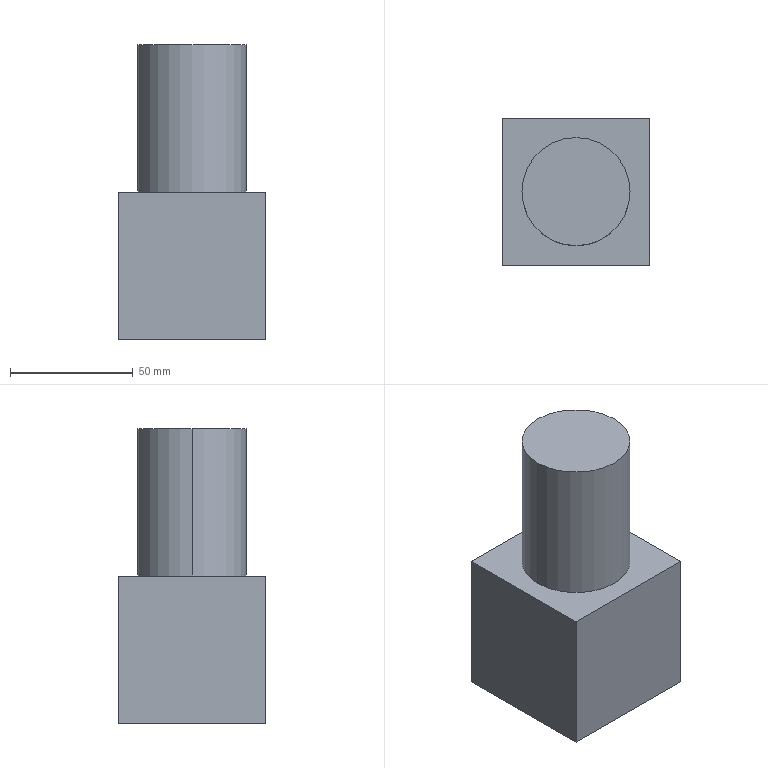Part | SolidWorks | features Extrusion 1, ICE 1 | 1 solid | 9 faces | box 60 x 60 x 120 mm | volume 307105 mm3 | plane 7 | cylinder 2 | commonest cylinder face diameters 43.97 x2
STEP:
#1=CARTESIAN_POINT('',(21.985,30.,90.));
#2=VERTEX_POINT('',#1);
#3=CARTESIAN_POINT('',(-21.985,30.,90.));
#4=VERTEX_POINT('',#3);
#5=CARTESIAN_POINT('',(0.,30.,90.));
#6=DIRECTION('',(0.,0.,1.));
#7=DIRECTION('',(1.,0.,0.));
#8=AXIS2_PLACEMENT_3D('',#5,#6,#7);
#9=CIRCLE('',#8,21.985);
#10=EDGE_CURVE('',#2,#4,#9,.T.);
#11=ORIENTED_EDGE('',*,*,#10,.F.);
#12=CARTESIAN_POINT('',(21.985,30.,30.));
#13=VERTEX_POINT('',#12);
#14=CARTESIAN_POINT('',(21.985,30.,90.));
#15=DIRECTION('',(0.,0.,-1.));
#16=VECTOR('',#15,1000.);
#17=LINE('',#14,#16);
#18=EDGE_CURVE('',#2,#13,#17,.T.);
#19=ORIENTED_EDGE('',*,*,#18,.T.);
#20=CARTESIAN_POINT('',(-21.985,30.,30.));
#21=VERTEX_POINT('',#20);
#22=CARTESIAN_POINT('',(0.,30.,30.));
#23=DIRECTION('',(0.,0.,1.));
#24=DIRECTION('',(1.,0.,0.));
#25=AXIS2_PLACEMENT_3D('',#22,#23,#24);
#26=CIRCLE('',#25,21.985);
#27=EDGE_CURVE('',#13,#21,#26,.T.);
#28=ORIENTED_EDGE('',*,*,#27,.T.);
#29=CARTESIAN_POINT('',(-21.985,30.,90.));
#30=DIRECTION('',(0.,0.,-1.));
#31=VECTOR('',#30,1000.);
#32=LINE('',#29,#31);
#33=EDGE_CURVE('',#4,#21,#32,.T.);
#34=ORIENTED_EDGE('',*,*,#33,.F.);
#35=EDGE_LOOP('',(#11,#19,#28,#34));
#36=FACE_OUTER_BOUND('',#35,.T.);
#37=CARTESIAN_POINT('',(0.,30.,90.));
#38=DIRECTION('',(0.,0.,-1.));
#39=DIRECTION('',(-1.,0.,0.));
#40=AXIS2_PLACEMENT_3D('',#37,#38,#39);
#41=CYLINDRICAL_SURFACE('',#40,21.985);
#42=ADVANCED_FACE('',(#36),#41,.T.);
#43=CARTESIAN_POINT('',(30.,0.,30.));
#44=VERTEX_POINT('',#43);
#45=CARTESIAN_POINT('',(30.,0.,-30.));
#46=VERTEX_POINT('',#45);
#47=CARTESIAN_POINT('',(30.,0.,-30.));
#48=DIRECTION('',(0.,0.,-1.));
#49=VECTOR('',#48,1000.);
#50=LINE('',#47,#49);
#51=EDGE_CURVE('',#44,#46,#50,.T.);
#52=ORIENTED_EDGE('',*,*,#51,.T.);
#53=CARTESIAN_POINT('',(30.,60.,-30.));
#54=VERTEX_POINT('',#53);
#55=CARTESIAN_POINT('',(30.,60.,-30.));
#56=DIRECTION('',(0.,-1.,0.));
#57=VECTOR('',#56,1000.);
#58=LINE('',#55,#57);
#59=EDGE_CURVE('',#54,#46,#58,.T.);
#60=ORIENTED_EDGE('',*,*,#59,.F.);
#61=CARTESIAN_POINT('',(30.,60.,30.));
#62=VERTEX_POINT('',#61);
#63=CARTESIAN_POINT('',(30.,60.,-30.));
#64=DIRECTION('',(0.,0.,-1.));
#65=VECTOR('',#64,1000.);
#66=LINE('',#63,#65);
#67=EDGE_CURVE('',#62,#54,#66,.T.);
#68=ORIENTED_EDGE('',*,*,#67,.F.);
#69=CARTESIAN_POINT('',(30.,60.,30.));
#70=DIRECTION('',(0.,-1.,0.));
#71=VECTOR('',#70,1000.);
#72=LINE('',#69,#71);
#73=EDGE_CURVE('',#62,#44,#72,.T.);
#74=ORIENTED_EDGE('',*,*,#73,.T.);
#75=EDGE_LOOP('',(#52,#60,#68,#74));
#76=FACE_OUTER_BOUND('',#75,.T.);
#77=CARTESIAN_POINT('',(30.,60.,-30.));
#78=DIRECTION('',(-1.,0.,0.));
#79=DIRECTION('',(0.,0.,1.));
#80=AXIS2_PLACEMENT_3D('',#77,#78,#79);
#81=PLANE('',#80);
#82=ADVANCED_FACE('',(#76),#81,.F.);
#83=CARTESIAN_POINT('',(-30.,0.,-30.));
#84=VERTEX_POINT('',#83);
#85=CARTESIAN_POINT('',(-30.,0.,-30.));
#86=DIRECTION('',(-1.,0.,0.));
#87=VECTOR('',#86,1000.);
#88=LINE('',#85,#87);
#89=EDGE_CURVE('',#46,#84,#88,.T.);
#90=ORIENTED_EDGE('',*,*,#89,.T.);
#91=CARTESIAN_POINT('',(-30.,60.,-30.));
#92=VERTEX_POINT('',#91);
#93=CARTESIAN_POINT('',(-30.,60.,-30.));
#94=DIRECTION('',(0.,-1.,0.));
#95=VECTOR('',#94,1000.);
#96=LINE('',#93,#95);
#97=EDGE_CURVE('',#92,#84,#96,.T.);
#98=ORIENTED_EDGE('',*,*,#97,.F.);
#99=CARTESIAN_POINT('',(-30.,60.,-30.));
#100=DIRECTION('',(-1.,0.,0.));
#101=VECTOR('',#100,1000.);
#102=LINE('',#99,#101);
#103=EDGE_CURVE('',#54,#92,#102,.T.);
#104=ORIENTED_EDGE('',*,*,#103,.F.);
#105=ORIENTED_EDGE('',*,*,#59,.T.);
#106=EDGE_LOOP('',(#90,#98,#104,#105));
#107=FACE_OUTER_BOUND('',#106,.T.);
#108=CARTESIAN_POINT('',(-30.,60.,-30.));
#109=DIRECTION('',(0.,0.,1.));
#110=DIRECTION('',(1.,0.,0.));
#111=AXIS2_PLACEMENT_3D('',#108,#109,#110);
#112=PLANE('',#111);
#113=ADVANCED_FACE('',(#107),#112,.F.);
#114=CARTESIAN_POINT('',(-30.,0.,30.));
#115=VERTEX_POINT('',#114);
#116=CARTESIAN_POINT('',(-30.,0.,-30.));
#117=DIRECTION('',(0.,0.,1.));
#118=VECTOR('',#117,1000.);
#119=LINE('',#116,#118);
#120=EDGE_CURVE('',#84,#115,#119,.T.);
#121=ORIENTED_EDGE('',*,*,#120,.T.);
#122=CARTESIAN_POINT('',(-30.,60.,30.));
#123=VERTEX_POINT('',#122);
#124=CARTESIAN_POINT('',(-30.,60.,30.));
#125=DIRECTION('',(0.,-1.,0.));
#126=VECTOR('',#125,1000.);
#127=LINE('',#124,#126);
#128=EDGE_CURVE('',#123,#115,#127,.T.);
#129=ORIENTED_EDGE('',*,*,#128,.F.);
#130=CARTESIAN_POINT('',(-30.,60.,-30.));
#131=DIRECTION('',(0.,0.,1.));
#132=VECTOR('',#131,1000.);
#133=LINE('',#130,#132);
#134=EDGE_CURVE('',#92,#123,#133,.T.);
#135=ORIENTED_EDGE('',*,*,#134,.F.);
#136=ORIENTED_EDGE('',*,*,#97,.T.);
#137=EDGE_LOOP('',(#121,#129,#135,#136));
#138=FACE_OUTER_BOUND('',#137,.T.);
#139=CARTESIAN_POINT('',(-30.,60.,-30.));
#140=DIRECTION('',(1.,0.,0.));
#141=DIRECTION('',(0.,0.,-1.));
#142=AXIS2_PLACEMENT_3D('',#139,#140,#141);
#143=PLANE('',#142);
#144=ADVANCED_FACE('',(#138),#143,.F.);
#145=CARTESIAN_POINT('',(0.,30.,30.));
#146=DIRECTION('',(0.,0.,1.));
#147=DIRECTION('',(1.,0.,0.));
#148=AXIS2_PLACEMENT_3D('',#145,#146,#147);
#149=CIRCLE('',#148,21.985);
#150=EDGE_CURVE('',#21,#13,#149,.T.);
#151=ORIENTED_EDGE('',*,*,#150,.F.);
#152=ORIENTED_EDGE('',*,*,#27,.F.);
#153=EDGE_LOOP('',(#151,#152));
#154=FACE_BOUND('',#153,.T.);
#155=CARTESIAN_POINT('',(-30.,0.,30.));
#156=DIRECTION('',(1.,0.,0.));
#157=VECTOR('',#156,1000.);
#158=LINE('',#155,#157);
#159=EDGE_CURVE('',#115,#44,#158,.T.);
#160=ORIENTED_EDGE('',*,*,#159,.T.);
#161=ORIENTED_EDGE('',*,*,#73,.F.);
#162=CARTESIAN_POINT('',(-30.,60.,30.));
#163=DIRECTION('',(1.,0.,0.));
#164=VECTOR('',#163,1000.);
#165=LINE('',#162,#164);
#166=EDGE_CURVE('',#123,#62,#165,.T.);
#167=ORIENTED_EDGE('',*,*,#166,.F.);
#168=ORIENTED_EDGE('',*,*,#128,.T.);
#169=EDGE_LOOP('',(#160,#161,#167,#168));
#170=FACE_OUTER_BOUND('',#169,.T.);
#171=CARTESIAN_POINT('',(-30.,60.,30.));
#172=DIRECTION('',(0.,0.,-1.));
#173=DIRECTION('',(-1.,0.,0.));
#174=AXIS2_PLACEMENT_3D('',#171,#172,#173);
#175=PLANE('',#174);
#176=ADVANCED_FACE('',(#154,#170),#175,.F.);
#177=ORIENTED_EDGE('',*,*,#67,.T.);
#178=ORIENTED_EDGE('',*,*,#103,.T.);
#179=ORIENTED_EDGE('',*,*,#134,.T.);
#180=ORIENTED_EDGE('',*,*,#166,.T.);
#181=EDGE_LOOP('',(#177,#178,#179,#180));
#182=FACE_OUTER_BOUND('',#181,.T.);
#183=CARTESIAN_POINT('',(0.,60.,0.));
#184=DIRECTION('',(0.,1.,0.));
#185=DIRECTION('',(0.,0.,1.));
#186=AXIS2_PLACEMENT_3D('',#183,#184,#185);
#187=PLANE('',#186);
#188=ADVANCED_FACE('',(#182),#187,.T.);
#189=ORIENTED_EDGE('',*,*,#51,.F.);
#190=ORIENTED_EDGE('',*,*,#159,.F.);
#191=ORIENTED_EDGE('',*,*,#120,.F.);
#192=ORIENTED_EDGE('',*,*,#89,.F.);
#193=EDGE_LOOP('',(#189,#190,#191,#192));
#194=FACE_OUTER_BOUND('',#193,.T.);
#195=CARTESIAN_POINT('',(0.,0.,0.));
#196=DIRECTION('',(0.,1.,0.));
#197=DIRECTION('',(0.,0.,1.));
#198=AXIS2_PLACEMENT_3D('',#195,#196,#197);
#199=PLANE('',#198);
#200=ADVANCED_FACE('',(#194),#199,.F.);
#201=ORIENTED_EDGE('',*,*,#18,.F.);
#202=CARTESIAN_POINT('',(0.,30.,90.));
#203=DIRECTION('',(0.,0.,1.));
#204=DIRECTION('',(1.,0.,0.));
#205=AXIS2_PLACEMENT_3D('',#202,#203,#204);
#206=CIRCLE('',#205,21.985);
#207=EDGE_CURVE('',#4,#2,#206,.T.);
#208=ORIENTED_EDGE('',*,*,#207,.F.);
#209=ORIENTED_EDGE('',*,*,#33,.T.);
#210=ORIENTED_EDGE('',*,*,#150,.T.);
#211=EDGE_LOOP('',(#201,#208,#209,#210));
#212=FACE_OUTER_BOUND('',#211,.T.);
#213=CARTESIAN_POINT('',(0.,30.,90.));
#214=DIRECTION('',(0.,0.,-1.));
#215=DIRECTION('',(-1.,0.,0.));
#216=AXIS2_PLACEMENT_3D('',#213,#214,#215);
#217=CYLINDRICAL_SURFACE('',#216,21.985);
#218=ADVANCED_FACE('',(#212),#217,.T.);
#219=ORIENTED_EDGE('',*,*,#207,.T.);
#220=ORIENTED_EDGE('',*,*,#10,.T.);
#221=EDGE_LOOP('',(#219,#220));
#222=FACE_OUTER_BOUND('',#221,.T.);
#223=CARTESIAN_POINT('',(0.,30.,90.));
#224=DIRECTION('',(0.,0.,1.));
#225=DIRECTION('',(1.,0.,0.));
#226=AXIS2_PLACEMENT_3D('',#223,#224,#225);
#227=PLANE('',#226);
#228=ADVANCED_FACE('',(#222),#227,.T.);
#229=CLOSED_SHELL('',(#42,#82,#113,#144,#176,#188,#200,#218,#228));
#230=MANIFOLD_SOLID_BREP('',#229);
#231=CARTESIAN_POINT('',(0.,0.,0.));
#232=DIRECTION('',(0.,0.,1.));
#233=DIRECTION('',(1.,0.,0.));
#234=AXIS2_PLACEMENT_3D('',#231,#232,#233);
#235=(LENGTH_UNIT()NAMED_UNIT(*)SI_UNIT(.MILLI.,.METRE.));
#236=UNCERTAINTY_MEASURE_WITH_UNIT(LENGTH_MEASURE(0.00001),#235,'','');
#237=(NAMED_UNIT(*)PLANE_ANGLE_UNIT()SI_UNIT($,.RADIAN.));
#238=(NAMED_UNIT(*)SI_UNIT($,.STERADIAN.)SOLID_ANGLE_UNIT());
#239=(GEOMETRIC_REPRESENTATION_CONTEXT(3)GLOBAL_UNCERTAINTY_ASSIGNED_CONTEXT((#236))GLOBAL_UNIT_ASSIGNED_CONTEXT((#235,#237,#238))REPRESENTATION_CONTEXT('',''));
#240=ADVANCED_BREP_SHAPE_REPRESENTATION('',(#230,#234),#239);